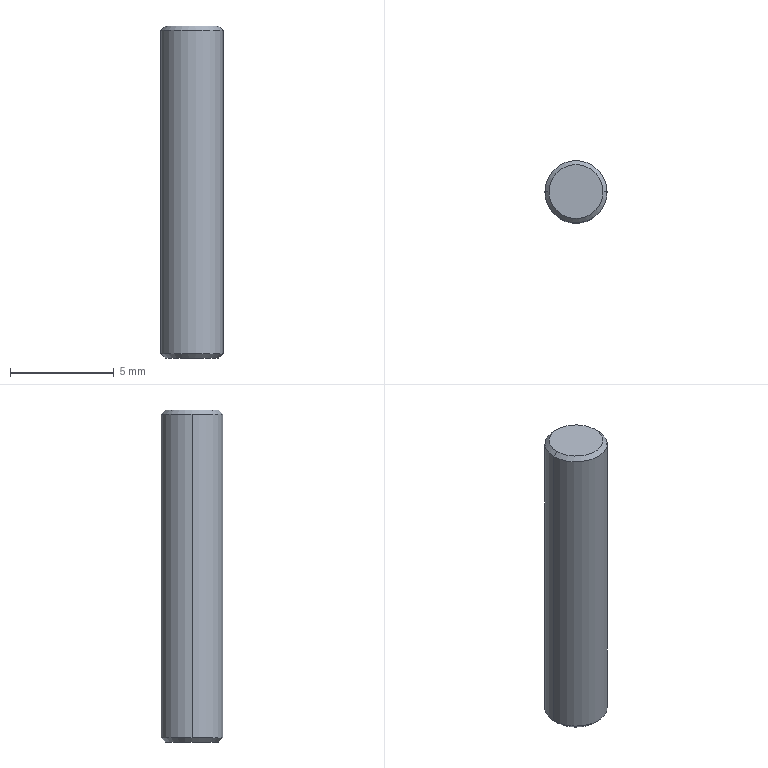Part | SolidWorks | features Chamfer 1, Extrusion 1 | 1 solid | 8 faces | box 3 x 3 x 16 mm | volume 112.737 mm3 | cone 4 | cylinder 2 | plane 2 | commonest cylinder face diameters 3 x2
STEP:
#1=CARTESIAN_POINT('',(1.3,0.,16.));
#2=VERTEX_POINT('',#1);
#3=CARTESIAN_POINT('',(-1.3,0.,16.));
#4=VERTEX_POINT('',#3);
#5=CARTESIAN_POINT('',(0.,0.,16.));
#6=DIRECTION('',(0.,0.,1.));
#7=DIRECTION('',(1.,0.,0.));
#8=AXIS2_PLACEMENT_3D('',#5,#6,#7);
#9=CIRCLE('',#8,1.3);
#10=EDGE_CURVE('',#2,#4,#9,.T.);
#11=ORIENTED_EDGE('',*,*,#10,.F.);
#12=CARTESIAN_POINT('',(1.5,0.,15.8));
#13=VERTEX_POINT('',#12);
#14=CARTESIAN_POINT('',(1.3,0.,16.));
#15=DIRECTION('',(0.7071,0.,-0.7071));
#16=VECTOR('',#15,1000.);
#17=LINE('',#14,#16);
#18=EDGE_CURVE('',#2,#13,#17,.T.);
#19=ORIENTED_EDGE('',*,*,#18,.T.);
#20=CARTESIAN_POINT('',(-1.5,0.,15.8));
#21=VERTEX_POINT('',#20);
#22=CARTESIAN_POINT('',(0.,0.,15.8));
#23=DIRECTION('',(0.,0.,-1.));
#24=DIRECTION('',(1.,0.,0.));
#25=AXIS2_PLACEMENT_3D('',#22,#23,#24);
#26=CIRCLE('',#25,1.5);
#27=EDGE_CURVE('',#21,#13,#26,.T.);
#28=ORIENTED_EDGE('',*,*,#27,.F.);
#29=CARTESIAN_POINT('',(-1.3,0.,16.));
#30=DIRECTION('',(-0.7071,0.,-0.7071));
#31=VECTOR('',#30,1000.);
#32=LINE('',#29,#31);
#33=EDGE_CURVE('',#4,#21,#32,.T.);
#34=ORIENTED_EDGE('',*,*,#33,.F.);
#35=EDGE_LOOP('',(#11,#19,#28,#34));
#36=FACE_OUTER_BOUND('',#35,.T.);
#37=CARTESIAN_POINT('',(0.,0.,16.));
#38=DIRECTION('',(0.,0.,-1.));
#39=DIRECTION('',(-1.,0.,0.));
#40=AXIS2_PLACEMENT_3D('',#37,#38,#39);
#41=CONICAL_SURFACE('',#40,1.3,0.7854);
#42=ADVANCED_FACE('',(#36),#41,.T.);
#43=CARTESIAN_POINT('',(-1.3,0.,0.));
#44=VERTEX_POINT('',#43);
#45=CARTESIAN_POINT('',(1.3,0.,0.));
#46=VERTEX_POINT('',#45);
#47=CARTESIAN_POINT('',(0.,0.,0.));
#48=DIRECTION('',(0.,0.,-1.));
#49=DIRECTION('',(1.,0.,0.));
#50=AXIS2_PLACEMENT_3D('',#47,#48,#49);
#51=CIRCLE('',#50,1.3);
#52=EDGE_CURVE('',#44,#46,#51,.T.);
#53=ORIENTED_EDGE('',*,*,#52,.F.);
#54=CARTESIAN_POINT('',(-1.5,0.,0.2));
#55=VERTEX_POINT('',#54);
#56=CARTESIAN_POINT('',(-1.5,0.,0.2));
#57=DIRECTION('',(-0.7071,0.,0.7071));
#58=VECTOR('',#57,1000.);
#59=LINE('',#56,#58);
#60=EDGE_CURVE('',#44,#55,#59,.T.);
#61=ORIENTED_EDGE('',*,*,#60,.T.);
#62=CARTESIAN_POINT('',(1.5,0.,0.2));
#63=VERTEX_POINT('',#62);
#64=CARTESIAN_POINT('',(0.,0.,0.2));
#65=DIRECTION('',(0.,0.,1.));
#66=DIRECTION('',(1.,0.,0.));
#67=AXIS2_PLACEMENT_3D('',#64,#65,#66);
#68=CIRCLE('',#67,1.5);
#69=EDGE_CURVE('',#63,#55,#68,.T.);
#70=ORIENTED_EDGE('',*,*,#69,.F.);
#71=CARTESIAN_POINT('',(1.5,0.,0.2));
#72=DIRECTION('',(0.7071,0.,0.7071));
#73=VECTOR('',#72,1000.);
#74=LINE('',#71,#73);
#75=EDGE_CURVE('',#46,#63,#74,.T.);
#76=ORIENTED_EDGE('',*,*,#75,.F.);
#77=EDGE_LOOP('',(#53,#61,#70,#76));
#78=FACE_OUTER_BOUND('',#77,.T.);
#79=CARTESIAN_POINT('',(0.,0.,0.2));
#80=DIRECTION('',(0.,0.,1.));
#81=DIRECTION('',(1.,0.,0.));
#82=AXIS2_PLACEMENT_3D('',#79,#80,#81);
#83=CONICAL_SURFACE('',#82,1.5,0.7854);
#84=ADVANCED_FACE('',(#78),#83,.T.);
#85=ORIENTED_EDGE('',*,*,#27,.T.);
#86=CARTESIAN_POINT('',(1.5,0.,16.));
#87=DIRECTION('',(0.,0.,-1.));
#88=VECTOR('',#87,1000.);
#89=LINE('',#86,#88);
#90=EDGE_CURVE('',#13,#63,#89,.T.);
#91=ORIENTED_EDGE('',*,*,#90,.T.);
#92=ORIENTED_EDGE('',*,*,#69,.T.);
#93=CARTESIAN_POINT('',(-1.5,0.,16.));
#94=DIRECTION('',(0.,0.,-1.));
#95=VECTOR('',#94,1000.);
#96=LINE('',#93,#95);
#97=EDGE_CURVE('',#21,#55,#96,.T.);
#98=ORIENTED_EDGE('',*,*,#97,.F.);
#99=EDGE_LOOP('',(#85,#91,#92,#98));
#100=FACE_OUTER_BOUND('',#99,.T.);
#101=CARTESIAN_POINT('',(0.,0.,16.));
#102=DIRECTION('',(0.,0.,-1.));
#103=DIRECTION('',(-1.,0.,0.));
#104=AXIS2_PLACEMENT_3D('',#101,#102,#103);
#105=CYLINDRICAL_SURFACE('',#104,1.5);
#106=ADVANCED_FACE('',(#100),#105,.T.);
#107=ORIENTED_EDGE('',*,*,#90,.F.);
#108=CARTESIAN_POINT('',(0.,0.,15.8));
#109=DIRECTION('',(0.,0.,-1.));
#110=DIRECTION('',(1.,0.,0.));
#111=AXIS2_PLACEMENT_3D('',#108,#109,#110);
#112=CIRCLE('',#111,1.5);
#113=EDGE_CURVE('',#13,#21,#112,.T.);
#114=ORIENTED_EDGE('',*,*,#113,.T.);
#115=ORIENTED_EDGE('',*,*,#97,.T.);
#116=CARTESIAN_POINT('',(0.,0.,0.2));
#117=DIRECTION('',(0.,0.,1.));
#118=DIRECTION('',(1.,0.,0.));
#119=AXIS2_PLACEMENT_3D('',#116,#117,#118);
#120=CIRCLE('',#119,1.5);
#121=EDGE_CURVE('',#55,#63,#120,.T.);
#122=ORIENTED_EDGE('',*,*,#121,.T.);
#123=EDGE_LOOP('',(#107,#114,#115,#122));
#124=FACE_OUTER_BOUND('',#123,.T.);
#125=CARTESIAN_POINT('',(0.,0.,16.));
#126=DIRECTION('',(0.,0.,-1.));
#127=DIRECTION('',(-1.,0.,0.));
#128=AXIS2_PLACEMENT_3D('',#125,#126,#127);
#129=CYLINDRICAL_SURFACE('',#128,1.5);
#130=ADVANCED_FACE('',(#124),#129,.T.);
#131=CARTESIAN_POINT('',(0.,0.,16.));
#132=DIRECTION('',(0.,0.,1.));
#133=DIRECTION('',(1.,0.,0.));
#134=AXIS2_PLACEMENT_3D('',#131,#132,#133);
#135=CIRCLE('',#134,1.3);
#136=EDGE_CURVE('',#4,#2,#135,.T.);
#137=ORIENTED_EDGE('',*,*,#136,.T.);
#138=ORIENTED_EDGE('',*,*,#10,.T.);
#139=EDGE_LOOP('',(#137,#138));
#140=FACE_OUTER_BOUND('',#139,.T.);
#141=CARTESIAN_POINT('',(0.,0.,16.));
#142=DIRECTION('',(0.,0.,1.));
#143=DIRECTION('',(1.,0.,0.));
#144=AXIS2_PLACEMENT_3D('',#141,#142,#143);
#145=PLANE('',#144);
#146=ADVANCED_FACE('',(#140),#145,.T.);
#147=CARTESIAN_POINT('',(0.,0.,0.));
#148=DIRECTION('',(0.,0.,-1.));
#149=DIRECTION('',(1.,0.,0.));
#150=AXIS2_PLACEMENT_3D('',#147,#148,#149);
#151=CIRCLE('',#150,1.3);
#152=EDGE_CURVE('',#46,#44,#151,.T.);
#153=ORIENTED_EDGE('',*,*,#152,.T.);
#154=ORIENTED_EDGE('',*,*,#52,.T.);
#155=EDGE_LOOP('',(#153,#154));
#156=FACE_OUTER_BOUND('',#155,.T.);
#157=CARTESIAN_POINT('',(0.,0.,0.));
#158=DIRECTION('',(0.,0.,1.));
#159=DIRECTION('',(1.,0.,0.));
#160=AXIS2_PLACEMENT_3D('',#157,#158,#159);
#161=PLANE('',#160);
#162=ADVANCED_FACE('',(#156),#161,.F.);
#163=ORIENTED_EDGE('',*,*,#60,.F.);
#164=ORIENTED_EDGE('',*,*,#152,.F.);
#165=ORIENTED_EDGE('',*,*,#75,.T.);
#166=ORIENTED_EDGE('',*,*,#121,.F.);
#167=EDGE_LOOP('',(#163,#164,#165,#166));
#168=FACE_OUTER_BOUND('',#167,.T.);
#169=CARTESIAN_POINT('',(0.,0.,0.2));
#170=DIRECTION('',(0.,0.,1.));
#171=DIRECTION('',(1.,0.,0.));
#172=AXIS2_PLACEMENT_3D('',#169,#170,#171);
#173=CONICAL_SURFACE('',#172,1.5,0.7854);
#174=ADVANCED_FACE('',(#168),#173,.T.);
#175=ORIENTED_EDGE('',*,*,#18,.F.);
#176=ORIENTED_EDGE('',*,*,#136,.F.);
#177=ORIENTED_EDGE('',*,*,#33,.T.);
#178=ORIENTED_EDGE('',*,*,#113,.F.);
#179=EDGE_LOOP('',(#175,#176,#177,#178));
#180=FACE_OUTER_BOUND('',#179,.T.);
#181=CARTESIAN_POINT('',(0.,0.,16.));
#182=DIRECTION('',(0.,0.,-1.));
#183=DIRECTION('',(-1.,0.,0.));
#184=AXIS2_PLACEMENT_3D('',#181,#182,#183);
#185=CONICAL_SURFACE('',#184,1.3,0.7854);
#186=ADVANCED_FACE('',(#180),#185,.T.);
#187=CLOSED_SHELL('',(#42,#84,#106,#130,#146,#162,#174,#186));
#188=MANIFOLD_SOLID_BREP('',#187);
#189=CARTESIAN_POINT('',(0.,0.,0.));
#190=DIRECTION('',(0.,0.,1.));
#191=DIRECTION('',(1.,0.,0.));
#192=AXIS2_PLACEMENT_3D('',#189,#190,#191);
#193=(LENGTH_UNIT()NAMED_UNIT(*)SI_UNIT(.MILLI.,.METRE.));
#194=UNCERTAINTY_MEASURE_WITH_UNIT(LENGTH_MEASURE(0.00001),#193,'','');
#195=(NAMED_UNIT(*)PLANE_ANGLE_UNIT()SI_UNIT($,.RADIAN.));
#196=(NAMED_UNIT(*)SI_UNIT($,.STERADIAN.)SOLID_ANGLE_UNIT());
#197=(GEOMETRIC_REPRESENTATION_CONTEXT(3)GLOBAL_UNCERTAINTY_ASSIGNED_CONTEXT((#194))GLOBAL_UNIT_ASSIGNED_CONTEXT((#193,#195,#196))REPRESENTATION_CONTEXT('',''));
#198=ADVANCED_BREP_SHAPE_REPRESENTATION('',(#188,#192),#197);